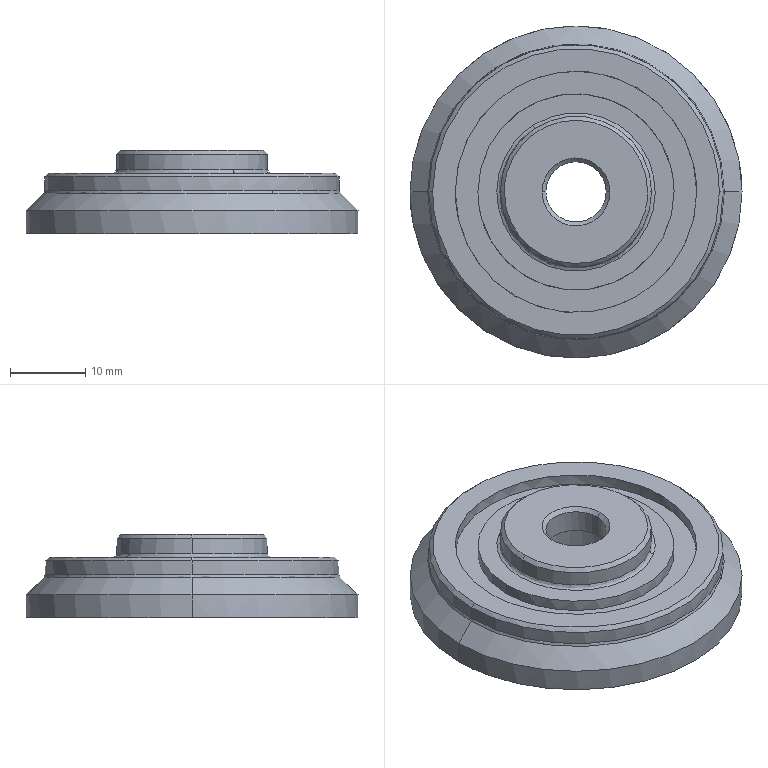Part | STEP file | Suporte Central-A | 1 solid | 38 faces | box 44 x 44 x 11 mm | volume 8128 mm3 | cylinder 18 | cone 8 | plane 8 | spline 4 | commonest cylinder face diameters 8 x2 15 x2 20 x2 26 x2 28 x2 32 x2